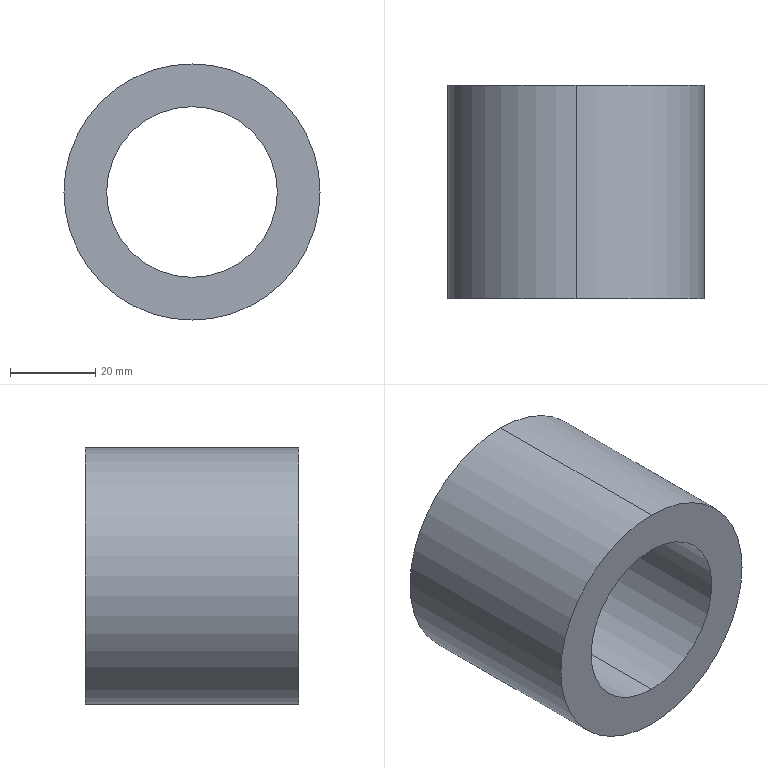Part | SolidWorks | features BaseBody 1 | 1 solid | 6 faces | box 60 x 50 x 60 mm | volume 78540 mm3 | cylinder 4 | plane 2 | commonest cylinder face diameters 40 x2 60 x2
STEP:
#1=CARTESIAN_POINT('',(0.,0.,30.));
#2=VERTEX_POINT('',#1);
#3=CARTESIAN_POINT('',(0.,0.,-30.));
#4=VERTEX_POINT('',#3);
#5=CARTESIAN_POINT('',(0.,0.,0.));
#6=DIRECTION('',(0.,1.,0.));
#7=DIRECTION('',(0.,0.,1.));
#8=AXIS2_PLACEMENT_3D('',#5,#6,#7);
#9=CIRCLE('',#8,30.);
#10=EDGE_CURVE('',#2,#4,#9,.T.);
#11=ORIENTED_EDGE('',*,*,#10,.T.);
#12=CARTESIAN_POINT('',(0.,50.,-30.));
#13=VERTEX_POINT('',#12);
#14=CARTESIAN_POINT('',(0.,0.,-30.));
#15=DIRECTION('',(0.,1.,0.));
#16=VECTOR('',#15,1000.);
#17=LINE('',#14,#16);
#18=EDGE_CURVE('',#4,#13,#17,.T.);
#19=ORIENTED_EDGE('',*,*,#18,.T.);
#20=CARTESIAN_POINT('',(0.,50.,30.));
#21=VERTEX_POINT('',#20);
#22=CARTESIAN_POINT('',(0.,50.,0.));
#23=DIRECTION('',(0.,-1.,0.));
#24=DIRECTION('',(0.,0.,1.));
#25=AXIS2_PLACEMENT_3D('',#22,#23,#24);
#26=CIRCLE('',#25,30.);
#27=EDGE_CURVE('',#13,#21,#26,.T.);
#28=ORIENTED_EDGE('',*,*,#27,.T.);
#29=CARTESIAN_POINT('',(0.,0.,30.));
#30=DIRECTION('',(0.,1.,0.));
#31=VECTOR('',#30,1000.);
#32=LINE('',#29,#31);
#33=EDGE_CURVE('',#2,#21,#32,.T.);
#34=ORIENTED_EDGE('',*,*,#33,.F.);
#35=EDGE_LOOP('',(#11,#19,#28,#34));
#36=FACE_OUTER_BOUND('',#35,.T.);
#37=CARTESIAN_POINT('',(0.,0.,0.));
#38=DIRECTION('',(0.,1.,0.));
#39=DIRECTION('',(0.,0.,1.));
#40=AXIS2_PLACEMENT_3D('',#37,#38,#39);
#41=CYLINDRICAL_SURFACE('',#40,30.);
#42=ADVANCED_FACE('',(#36),#41,.T.);
#43=CARTESIAN_POINT('',(0.,0.,20.));
#44=VERTEX_POINT('',#43);
#45=CARTESIAN_POINT('',(0.,0.,-20.));
#46=VERTEX_POINT('',#45);
#47=CARTESIAN_POINT('',(0.,0.,0.));
#48=DIRECTION('',(0.,-1.,0.));
#49=DIRECTION('',(0.,0.,1.));
#50=AXIS2_PLACEMENT_3D('',#47,#48,#49);
#51=CIRCLE('',#50,20.);
#52=EDGE_CURVE('',#44,#46,#51,.T.);
#53=ORIENTED_EDGE('',*,*,#52,.T.);
#54=CARTESIAN_POINT('',(0.,50.,-20.));
#55=VERTEX_POINT('',#54);
#56=CARTESIAN_POINT('',(0.,0.,-20.));
#57=DIRECTION('',(0.,1.,0.));
#58=VECTOR('',#57,1000.);
#59=LINE('',#56,#58);
#60=EDGE_CURVE('',#46,#55,#59,.T.);
#61=ORIENTED_EDGE('',*,*,#60,.T.);
#62=CARTESIAN_POINT('',(0.,50.,20.));
#63=VERTEX_POINT('',#62);
#64=CARTESIAN_POINT('',(0.,50.,0.));
#65=DIRECTION('',(0.,-1.,0.));
#66=DIRECTION('',(0.,0.,1.));
#67=AXIS2_PLACEMENT_3D('',#64,#65,#66);
#68=CIRCLE('',#67,20.);
#69=EDGE_CURVE('',#63,#55,#68,.T.);
#70=ORIENTED_EDGE('',*,*,#69,.F.);
#71=CARTESIAN_POINT('',(0.,0.,20.));
#72=DIRECTION('',(0.,1.,0.));
#73=VECTOR('',#72,1000.);
#74=LINE('',#71,#73);
#75=EDGE_CURVE('',#44,#63,#74,.T.);
#76=ORIENTED_EDGE('',*,*,#75,.F.);
#77=EDGE_LOOP('',(#53,#61,#70,#76));
#78=FACE_OUTER_BOUND('',#77,.T.);
#79=CARTESIAN_POINT('',(0.,0.,0.));
#80=DIRECTION('',(0.,1.,0.));
#81=DIRECTION('',(0.,0.,1.));
#82=AXIS2_PLACEMENT_3D('',#79,#80,#81);
#83=CYLINDRICAL_SURFACE('',#82,20.);
#84=ADVANCED_FACE('',(#78),#83,.F.);
#85=ORIENTED_EDGE('',*,*,#18,.F.);
#86=CARTESIAN_POINT('',(0.,0.,0.));
#87=DIRECTION('',(0.,1.,0.));
#88=DIRECTION('',(0.,0.,1.));
#89=AXIS2_PLACEMENT_3D('',#86,#87,#88);
#90=CIRCLE('',#89,30.);
#91=EDGE_CURVE('',#4,#2,#90,.T.);
#92=ORIENTED_EDGE('',*,*,#91,.T.);
#93=ORIENTED_EDGE('',*,*,#33,.T.);
#94=CARTESIAN_POINT('',(0.,50.,0.));
#95=DIRECTION('',(0.,-1.,0.));
#96=DIRECTION('',(0.,0.,1.));
#97=AXIS2_PLACEMENT_3D('',#94,#95,#96);
#98=CIRCLE('',#97,30.);
#99=EDGE_CURVE('',#21,#13,#98,.T.);
#100=ORIENTED_EDGE('',*,*,#99,.T.);
#101=EDGE_LOOP('',(#85,#92,#93,#100));
#102=FACE_OUTER_BOUND('',#101,.T.);
#103=CARTESIAN_POINT('',(0.,0.,0.));
#104=DIRECTION('',(0.,1.,0.));
#105=DIRECTION('',(0.,0.,1.));
#106=AXIS2_PLACEMENT_3D('',#103,#104,#105);
#107=CYLINDRICAL_SURFACE('',#106,30.);
#108=ADVANCED_FACE('',(#102),#107,.T.);
#109=ORIENTED_EDGE('',*,*,#52,.F.);
#110=CARTESIAN_POINT('',(0.,0.,0.));
#111=DIRECTION('',(0.,-1.,0.));
#112=DIRECTION('',(0.,0.,1.));
#113=AXIS2_PLACEMENT_3D('',#110,#111,#112);
#114=CIRCLE('',#113,20.);
#115=EDGE_CURVE('',#46,#44,#114,.T.);
#116=ORIENTED_EDGE('',*,*,#115,.F.);
#117=EDGE_LOOP('',(#109,#116));
#118=FACE_BOUND('',#117,.T.);
#119=ORIENTED_EDGE('',*,*,#10,.F.);
#120=ORIENTED_EDGE('',*,*,#91,.F.);
#121=EDGE_LOOP('',(#119,#120));
#122=FACE_OUTER_BOUND('',#121,.T.);
#123=CARTESIAN_POINT('',(0.,0.,0.));
#124=DIRECTION('',(0.,1.,0.));
#125=DIRECTION('',(0.,0.,1.));
#126=AXIS2_PLACEMENT_3D('',#123,#124,#125);
#127=PLANE('',#126);
#128=ADVANCED_FACE('',(#118,#122),#127,.F.);
#129=ORIENTED_EDGE('',*,*,#69,.T.);
#130=CARTESIAN_POINT('',(0.,50.,0.));
#131=DIRECTION('',(0.,-1.,0.));
#132=DIRECTION('',(0.,0.,1.));
#133=AXIS2_PLACEMENT_3D('',#130,#131,#132);
#134=CIRCLE('',#133,20.);
#135=EDGE_CURVE('',#55,#63,#134,.T.);
#136=ORIENTED_EDGE('',*,*,#135,.T.);
#137=EDGE_LOOP('',(#129,#136));
#138=FACE_BOUND('',#137,.T.);
#139=ORIENTED_EDGE('',*,*,#99,.F.);
#140=ORIENTED_EDGE('',*,*,#27,.F.);
#141=EDGE_LOOP('',(#139,#140));
#142=FACE_OUTER_BOUND('',#141,.T.);
#143=CARTESIAN_POINT('',(0.,50.,0.));
#144=DIRECTION('',(0.,1.,0.));
#145=DIRECTION('',(0.,0.,1.));
#146=AXIS2_PLACEMENT_3D('',#143,#144,#145);
#147=PLANE('',#146);
#148=ADVANCED_FACE('',(#138,#142),#147,.T.);
#149=ORIENTED_EDGE('',*,*,#60,.F.);
#150=ORIENTED_EDGE('',*,*,#115,.T.);
#151=ORIENTED_EDGE('',*,*,#75,.T.);
#152=ORIENTED_EDGE('',*,*,#135,.F.);
#153=EDGE_LOOP('',(#149,#150,#151,#152));
#154=FACE_OUTER_BOUND('',#153,.T.);
#155=CARTESIAN_POINT('',(0.,0.,0.));
#156=DIRECTION('',(0.,1.,0.));
#157=DIRECTION('',(0.,0.,1.));
#158=AXIS2_PLACEMENT_3D('',#155,#156,#157);
#159=CYLINDRICAL_SURFACE('',#158,20.);
#160=ADVANCED_FACE('',(#154),#159,.F.);
#161=CLOSED_SHELL('',(#42,#84,#108,#128,#148,#160));
#162=MANIFOLD_SOLID_BREP('',#161);
#163=CARTESIAN_POINT('',(0.,0.,0.));
#164=DIRECTION('',(0.,0.,1.));
#165=DIRECTION('',(1.,0.,0.));
#166=AXIS2_PLACEMENT_3D('',#163,#164,#165);
#167=(LENGTH_UNIT()NAMED_UNIT(*)SI_UNIT(.MILLI.,.METRE.));
#168=UNCERTAINTY_MEASURE_WITH_UNIT(LENGTH_MEASURE(0.00001),#167,'','');
#169=(NAMED_UNIT(*)PLANE_ANGLE_UNIT()SI_UNIT($,.RADIAN.));
#170=(NAMED_UNIT(*)SI_UNIT($,.STERADIAN.)SOLID_ANGLE_UNIT());
#171=(GEOMETRIC_REPRESENTATION_CONTEXT(3)GLOBAL_UNCERTAINTY_ASSIGNED_CONTEXT((#168))GLOBAL_UNIT_ASSIGNED_CONTEXT((#167,#169,#170))REPRESENTATION_CONTEXT('',''));
#172=ADVANCED_BREP_SHAPE_REPRESENTATION('',(#162,#166),#171);